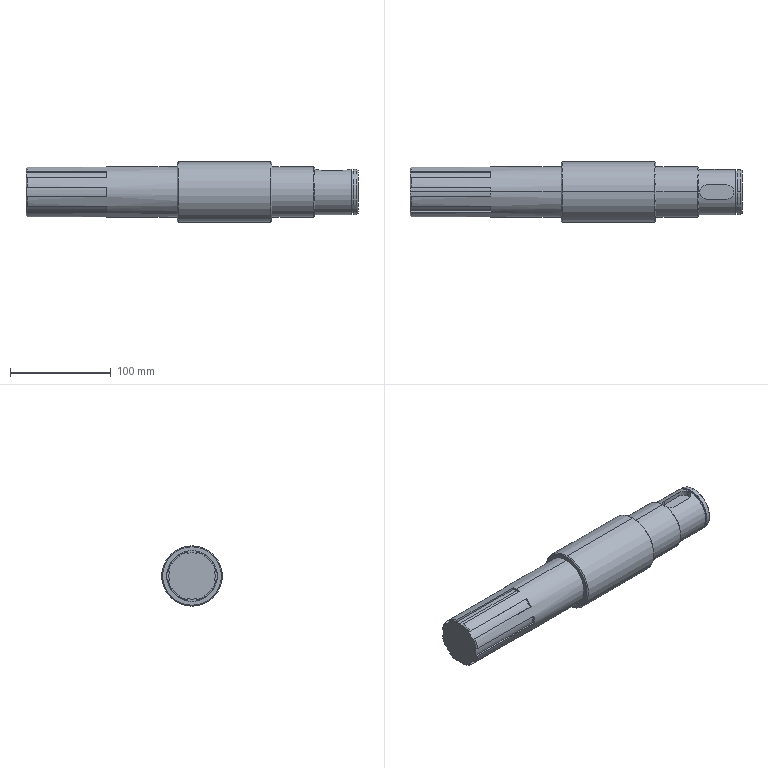Part | SolidWorks | features ICE 3, Chamfer 2, Revolution 1 | 1 solid | 74 faces | box 329.5 x 60 x 60 mm | volume 697643 mm3 | plane 34 | cylinder 24 | cone 16 | commonest cylinder face diameters 46 x9 45 x4 50 x4 14 x3 42.5 x2 60 x2